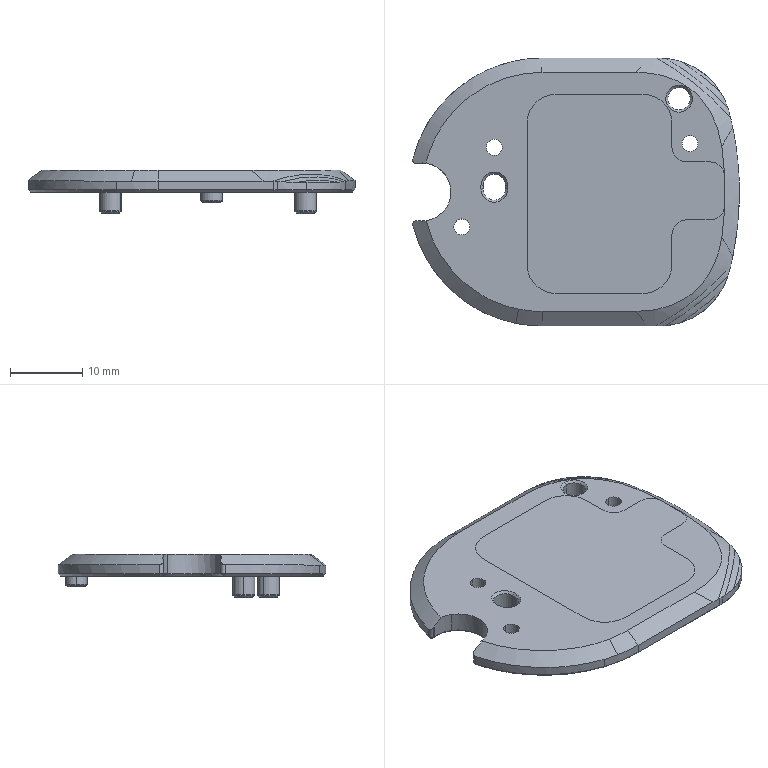NC program | NX | posted with a generic post | part box 45.101 x 36.973 x 6 mm
Lines 1809 to 2742 of 5084:
(ZLEVEL_PROFILE_1_COPY , TOOL : D3R0.5)
N3586 T18 M6
N3588 G54
N3590 G17 G0 G90 X-12.226 Y-12.18 S9500 M3
N3592 G43 Z30. H18
N3594 Z-2.01
N3596 G94 G1 Z-3.01 F1000.
N3598 X-12.477 Y-11.826
N3600 G3 X-12.75 Y-11.7 R0.3
N3602 G1 X-13.561 Y-11.776 F3000.
N3604 X-14.695 Y-11.793
N3606 X-14.752 Y-11.761
N3608 X-14.704 Y-12.064
N3610 X-14.705 Y-16.143
N3612 X-5.599 Y-16.003
N3614 G3 X-5.335 Y-15.728 R0.269
N3616 G1 X-5.334 Y-14.398
N3618 X-5.255 Y-13.594
N3620 X-5.37 Y-13.595 Z-3.019
N3622 X-5.415 Z-3.028
N3624 X-5.432 Y-14.398
N3626 Y-15.733
N3628 G2 X-5.601 Y-15.906 R0.171
N3630 G1 X-14.612 Y-16.044
N3632 X-14.608 Y-15.877
N3634 X-14.607 Y-12.131
N3636 X-14.614 Y-11.889
N3638 X-13.551 Y-11.873
N3640 X-12.739 Y-11.822
N3642 X-12.732 Y-11.89 Z-3.042
N3644 X-12.727 Y-11.939 Z-3.057
N3646 X-13.418 Y-11.959
N3648 X-13.54 Y-11.969
N3650 X-14.511 Y-11.984
N3652 X-14.512 Y-15.947
N3654 X-5.602 Y-15.81
N3656 X-5.56 Y-15.809
N3658 X-5.53 Y-15.778
N3660 X-5.528 Y-15.736
N3662 Y-14.398
N3664 X-5.509 Y-13.594
N3666 X-5.558 Y-13.595 Z-3.075
N3668 X-5.597 Z-3.094
N3670 X-5.619 Y-14.398
N3672 Y-15.719
N3674 X-14.42 Y-15.854
N3676 Y-12.074
N3678 X-13.529 Y-12.06
N3680 X-12.718 Y-12.035
N3682 X-12.712 Y-12.08 Z-3.117
N3684 X-12.707 Y-12.126 Z-3.139
N3686 X-13.418 Y-12.14
N3688 X-13.518 Y-12.146
N3690 X-14.333 Y-12.159
N3692 X-14.334 Y-15.766
N3694 X-5.706 Y-15.634
N3696 Y-14.398
N3698 X-5.686 Y-13.597
N3700 X-5.728 Z-3.166
N3702 X-5.772 Z-3.193
N3704 X-5.787 Y-14.398
N3706 Y-15.554
N3708 X-14.253 Y-15.684
N3710 X-14.252 Y-12.239
N3712 X-13.507 Y-12.227
N3714 X-12.697 Y-12.203
N3716 X-12.692 Y-12.246 Z-3.224
N3718 X-12.688 Y-12.283 Z-3.255
N3720 X-13.418 Y-12.296
N3722 X-13.496 Y-12.304
N3724 X-14.175 Y-12.315
N3726 X-14.176 Y-15.606
N3728 X-5.864 Y-15.478
N3730 Y-14.398
N3732 X-5.855 Y-14.33
N3734 X-5.844 Y-13.598
N3736 X-5.884 Z-3.29
N3738 X-5.917 Z-3.325
N3740 G2 X-5.934 Y-14.398 R6.646
N3742 G1 Y-15.409
N3744 X-14.105 Y-15.534
N3746 Y-12.384
N3748 X-13.485 Y-12.375
N3750 X-13.418 Y-12.371
N3752 X-12.679 Y-12.352
N3754 X-12.67 Y-12.39 Z-3.364
N3756 X-12.665 Y-12.412 Z-3.402
N3758 G3 X-13.475 Y-12.438 R18.194
N3760 G1 X-14.041 Y-12.447
N3762 Y-15.469
N3764 X-5.998 Y-15.346
N3766 Y-14.398
N3768 G3 X-5.981 Y-13.598 R6.688
N3770 G1 X-6.016 Z-3.444
N3772 X-6.044 Z-3.485
N3774 X-6.047 Y-14.33
N3776 X-6.053 Y-14.398
N3778 X-6.054 Y-15.291
N3780 X-13.986 Y-15.413
N3782 Y-12.501
N3784 X-13.466 Y-12.493
N3786 X-12.649 Y-12.469
N3788 X-12.633 Y-12.52 Z-3.571
N3790 X-12.69 Y-12.524
N3792 X-13.445 Y-12.536
N3794 X-13.458 Y-12.539
N3796 X-13.939 Y-12.547
N3798 X-13.94 Y-15.366
N3800 X-6.1 Y-15.246
N3802 Y-14.398
N3804 X-6.096 Y-14.33
N3806 Y-13.598
N3808 X-6.116 Z-3.614
N3810 X-6.138 Z-3.657
N3812 X-6.137 Y-14.33
N3814 X-6.135 Y-14.398
N3816 X-6.136 Y-15.211
N3818 X-13.904 Y-15.33
N3820 Y-12.582
N3822 X-13.451 Y-12.575
N3824 X-13.435 Y-12.577
N3826 X-12.69 Y-12.568
N3828 X-12.618 Y-12.564
N3830 X-12.603 Y-12.606 Z-3.738
N3832 X-12.69 Y-12.61
N3834 X-13.418 Y-12.617
N3836 X-13.429 Y-12.614
N3838 X-13.878 Y-12.621
N3840 Y-15.29
N3842 X-6.175 Y-15.172
N3844 Y-14.398
N3846 X-6.182 Y-14.33
N3848 X-6.183 Y-13.598
N3850 X-6.204 Z-3.768
N3852 X-6.224 Z-3.798
N3854 Y-14.33
N3856 X-6.217 Y-14.398
N3858 X-6.218 Y-15.13
N3860 X-13.864 Y-15.247
N3862 X-13.863 Y-12.663
N3864 X-13.405 Y-12.656
N3866 X-12.564 Y-12.649
N3868 X-12.508 Y-12.706 Z-3.859
N3870 X-13.371 Y-12.715
N3872 X-13.853 Y-12.723
N3874 Y-15.188
N3876 X-6.277 Y-15.071
N3878 Y-14.398
N3880 X-6.285 Y-14.33
N3882 Y-13.598
N3884 X-6.325 Z-3.886
N3886 X-6.367 Z-3.914
N3888 Y-14.33
N3890 X-6.355 Y-14.398
N3892 Y-14.995
N3894 X-13.847 Y-15.11
N3896 Y-12.8
N3898 X-13.323 Y-12.792
N3900 X-12.458 Y-12.786
N3902 X-12.351 Y-12.802 Z-3.926
N3904 X-12.243 Y-12.823 Z-3.938
N3906 X-12.136 Y-12.841 Z-3.951
N3908 X-12.222 Y-12.855
N3910 X-12.361 Y-12.869
N3912 X-12.448 Y-12.875
N3914 X-13.175 Y-12.889
N3916 X-13.265 Y-12.872
N3918 X-13.844 Y-12.881
N3920 Y-15.029
N3922 X-6.435 Y-14.916
N3924 Y-14.398
N3926 X-6.461 Y-14.33
N3928 X-6.45 Y-13.598
N3930 X-6.529 Y-13.602 Z-3.969
N3932 X-6.534 Y-14.33
N3934 X-6.5 Y-14.398
N3936 Y-14.851
N3938 X-13.844 Y-14.964
N3940 X-13.843 Y-12.946
N3942 X-13.213 Y-12.936
N3944 X-12.283 Y-12.95
N3946 G3 X-11.734 Y-12.785 R1.156
N3948 G1 X-11.72 Y-12.773
N3950 X-11.582 Y-12.722
N3952 X-11.587 Y-12.703
N3954 X-11.504 Y-12.759 Z-3.98
N3956 G2 X-12.142 Y-13.022 R0.839
N3958 G1 X-13.167 Y-12.989
N3960 X-13.843 Y-12.999
N3962 Y-14.911
N3964 X-6.553 Y-14.799
N3966 Y-14.398
N3968 G2 X-6.591 Y-13.594 R5.438
N3970 G3 X-6.734 Y-13.33 R0.3
N3972 G1 X-7.105 Y-13.103
N3974 Z-2.98
N3976 G0 Z30.
(ZLEVEL_PROFILE_1_COPY_COPY , TOOL : D3R0.5)
N3978 X11.743 Y-13.383
N3980 Z0.98
N3982 G1 Z-0.02 F1000.
N3984 X11.508 Y-12.976
N3986 G3 X11.248 Y-12.826 R0.3
N3988 G2 X8.967 Y-10.544 R2.282 F3000.
N3990 X11.248 Y-12.826 R-2.282
N3992 G1 Y-12.883 Z-0.036
N3994 Y-12.928 Z-0.053
N3996 G3 X13.632 Y-10.544 R2.384
N3998 X11.248 Y-12.928 R-2.384
N4000 G1 Y-12.978 Z-0.076
N4002 Y-13.02 Z-0.099
N4004 G2 X8.772 Y-10.544 R2.476
N4006 X11.248 Y-13.02 R-2.476
N4008 G1 Y-13.065 Z-0.128
N4010 Y-13.103 Z-0.157
N4012 G3 X13.808 Y-10.544 R2.559
N4014 X11.248 Y-13.103 R-2.559
N4016 G1 Y-13.142 Z-0.192
N4018 Y-13.177 Z-0.226
N4020 G2 X8.615 Y-10.544 R2.633
N4022 X11.248 Y-13.177 R-2.633
N4024 G1 Y-13.248 Z-0.297
N4026 G3 X13.952 Y-10.544 R2.704
N4028 X11.248 Y-13.248 R-2.704
N4030 G1 Y-13.318 Z-0.367
N4032 G2 X8.474 Y-10.544 R2.774
N4034 X11.248 Y-13.318 R-2.774
N4036 G1 Y-13.355 Z-0.404
N4038 Y-13.387 Z-0.441
N4040 G3 X14.091 Y-10.544 R2.843
N4042 X11.248 Y-13.387 R-2.843
N4044 G1 Y-13.418 Z-0.482
N4046 Y-13.445 Z-0.523
N4048 G2 X8.348 Y-10.544 R2.901
N4050 X11.248 Y-13.445 R-2.901
N4052 G1 Y-13.464 Z-0.558
N4054 Y-13.481 Z-0.593
N4056 G3 X14.185 Y-10.544 R2.937
N4058 X11.248 Y-13.481 R-2.937
N4060 G1 Y-13.495 Z-0.627
N4062 Y-13.508 Z-0.662
N4064 G2 X8.284 Y-10.544 R2.964
N4066 X11.248 Y-13.508 R-2.964
N4068 G1 Y-13.519 Z-0.696
N4070 Y-13.527 Z-0.731
N4072 G3 X14.232 Y-10.544 R2.983
N4074 X11.248 Y-13.527 R-2.983
N4076 G1 Y-13.534 Z-0.765
N4078 Y-13.539 Z-0.8
N4080 G2 X8.253 Y-10.544 R2.995
N4082 X11.248 Y-13.539 R-2.995
N4084 G3 X10.989 Y-13.689 R0.3
N4086 G1 X10.749 Y-14.104
N4088 Z0.2
N4090 G0 Z30.
N4092 X-18.519 Y-7.637
N4094 Z0.98
N4096 G1 Z-0.02 F1000.
N4098 X-18.111 Y-7.402
N4100 G3 X-17.961 Y-7.142 R0.3
N4102 G2 X-15.679 Y-4.86 R2.282 F3000.
N4104 X-17.961 Y-7.142 R-2.282
N4106 G1 X-18.019 Z-0.036
N4108 X-18.064 Z-0.053
N4110 G3 X-15.679 Y-9.526 R2.384
N4112 X-18.064 Y-7.142 R-2.384
N4114 G1 X-18.114 Z-0.076
N4116 X-18.156 Z-0.099
N4118 G2 X-15.679 Y-4.666 R2.476
N4120 X-18.156 Y-7.142 R-2.476
N4122 G1 X-18.2 Z-0.128
N4124 X-18.239 Z-0.157
N4126 G3 X-15.679 Y-9.702 R2.559
N4128 X-18.239 Y-7.142 R-2.559
N4130 G1 X-18.278 Z-0.192
N4132 X-18.313 Z-0.226
N4134 G2 X-15.679 Y-4.509 R2.633
N4136 X-18.313 Y-7.142 R-2.633
N4138 G1 X-18.383 Z-0.297
N4140 G3 X-15.679 Y-9.846 R2.704
N4142 X-18.383 Y-7.142 R-2.704
N4144 G1 X-18.454 Z-0.367
N4146 G2 X-15.679 Y-4.368 R2.775
N4148 X-18.454 Y-7.142 R-2.775
N4150 G1 X-18.49 Z-0.404
N4152 X-18.523 Z-0.441
N4154 G3 X-15.679 Y-9.985 R2.843
N4156 X-18.523 Y-7.142 R-2.843
N4158 G1 X-18.554 Z-0.482
N4160 X-18.58 Z-0.523
N4162 G2 X-15.679 Y-4.241 R2.901
N4164 X-18.58 Y-7.142 R-2.901
N4166 G1 X-18.6 Z-0.558
N4168 X-18.617 Z-0.593
N4170 G3 X-15.679 Y-10.079 R2.937
N4172 X-18.617 Y-7.142 R-2.937
N4174 G1 X-18.631 Z-0.627
N4176 X-18.644 Z-0.662
N4178 G2 X-15.679 Y-4.178 R2.964
N4180 X-18.644 Y-7.142 R-2.964
N4182 G1 X-18.654 Z-0.696
N4184 X-18.663 Z-0.731
N4186 G3 X-15.679 Y-10.126 R2.983
N4188 X-18.663 Y-7.142 R-2.983
N4190 G1 X-18.67 Z-0.765
N4192 X-18.675 Z-0.8
N4194 G2 X-15.679 Y-4.147 R2.995
N4196 X-18.675 Y-7.142 R-2.995
N4198 G3 X-18.825 Y-6.882 R0.3
N4200 G1 X-19.24 Y-6.643
N4202 Z0.2
N4204 G0 Z30.
(ZLEVEL_PROFILE_1_COPY_COPY_COPY , TOOL : D3R0.5)
N4206 X-3.201 Y18.824
N4208 Z-0.52
N4210 G1 Z-1.52 F1000.
N4212 X-2.966 Y18.417
N4214 G3 X-2.707 Y18.267 R0.3
N4216 G2 X-0.425 Y15.985 R2.282 F3000.
N4218 X-2.707 Y18.267 R-2.282
N4220 G1 Y18.324 Z-1.536
N4222 Y18.369 Z-1.553
N4224 G3 X-5.091 Y15.985 R2.384
N4226 X-2.707 Y18.369 R-2.384
N4228 G1 Y18.419 Z-1.576
N4230 Y18.461 Z-1.599
N4232 G2 X-0.231 Y15.985 R2.476
N4234 X-2.707 Y18.461 R-2.476
N4236 G1 Y18.506 Z-1.628
N4238 Y18.544 Z-1.657
N4240 G3 X-5.266 Y15.985 R2.559
N4242 X-2.707 Y18.544 R-2.559
N4244 G1 Y18.583 Z-1.692
N4246 Y18.618 Z-1.726
N4248 G2 X-0.074 Y15.985 R2.633
N4250 X-2.707 Y18.618 R-2.633
N4252 G1 Y18.689 Z-1.797
N4254 G3 X-5.41 Y15.985 R2.704
N4256 X-2.707 Y18.689 R-2.704
N4258 G1 Y18.759 Z-1.867
N4260 G2 X0.068 Y15.985 R2.774
N4262 X-2.707 Y18.759 R-2.774
N4264 G1 Y18.796 Z-1.904
N4266 Y18.828 Z-1.941
N4268 G3 X-5.55 Y15.985 R2.843
N4270 X-2.707 Y18.828 R-2.843
N4272 G1 Y18.859 Z-1.982
N4274 Y18.886 Z-2.023
N4276 G2 X0.194 Y15.985 R2.901
N4278 X-2.707 Y18.886 R-2.901
N4280 G1 Y18.905 Z-2.058
N4282 Y18.922 Z-2.093
N4284 G3 X-5.644 Y15.985 R2.937
N4286 X-2.707 Y18.922 R-2.937
N4288 G1 Y18.937 Z-2.127
N4290 Y18.949 Z-2.162
N4292 G2 X0.258 Y15.985 R2.964
N4294 X-2.707 Y18.949 R-2.964
N4296 G1 Y18.96 Z-2.196
N4298 Y18.968 Z-2.231
N4300 G3 X-5.69 Y15.985 R2.983
N4302 X-2.707 Y18.968 R-2.983
N4304 G1 Y18.975 Z-2.265
N4306 Y18.98 Z-2.3
N4308 G2 X0.289 Y15.985 R2.995
N4310 X-2.707 Y18.98 R-2.995
N4312 G3 X-2.447 Y19.13 R0.3
N4314 G1 X-2.207 Y19.545
N4316 Z-1.3
N4318 G0 Z30.
(FIXED_CONTOUR , TOOL : D3R0.5)
N4320 X-12.11 Y-12.283
N4322 Z0.
N4324 G1 Z-3.651 F1000.
N4326 G2 X-12.234 Y-12.01 R0.3
N4328 G1 X-12.229 Y-11.962 Z-3.584 F2500.
N4330 X-12.201 Y-11.849 Z-3.494
N4332 X-12.145 Y-11.593 Z-3.363
N4334 X-12.132 Y-11.319 Z-3.254
N4336 X-12.149 Y-11.088 Z-3.182
N4338 X-12.19 Y-10.835 Z-3.124
N4340 X-12.25 Y-10.577 Z-3.086
N4342 X-12.295 Y-10.368 Z-3.077
N4344 X-12.296 Y-9.711 Z-3.086
N4346 Y-8.106
N4348 Y-6.502
N4350 X-12.292 Y-6.1 Z-3.088
N4352 X-12.295 Y-5.541 Z-3.096
N4354 X-12.362 Y-5.173 Z-3.093
N4356 X-12.473 Y-4.819 Z-3.09
N4358 X-12.626 Y-4.482 Z-3.089
N4360 X-12.82 Y-4.166 Z-3.087
N4362 X-13.051 Y-3.875
N4364 X-13.318 Y-3.613 Z-3.086
N4366 X-13.613 Y-3.389 Z-3.087
N4368 X-13.931 Y-3.203 Z-3.088
N4370 X-14.269 Y-3.057 Z-3.089
N4372 X-14.624 Y-2.953 Z-3.091
N4374 X-14.99 Y-2.893 Z-3.093
N4376 X-15.325 Y-2.882
N4378 X-16.93 Y-2.894 Z-3.086
N4380 X-18.534
N4382 X-18.717 Y-2.893 Z-3.077
N4384 X-18.881 Y-2.841 Z-3.079
N4386 X-19.034 Y-2.765 Z-3.082
N4388 X-19.173 Y-2.666 Z-3.084
N4390 X-19.296 Y-2.546 Z-3.085
N4392 X-19.398 Y-2.409 Z-3.086
N4394 X-19.476 Y-2.258
N4396 X-19.53 Y-2.097
N4398 X-19.559 Y-1.929 Z-3.085
N4400 X-19.56 Y-1.619 Z-3.086
N4402 Y-0.817
N4404 Y0.788
N4406 X-19.559 Y1.59
N4408 X-19.556 Y2.252
N4410 X-19.527 Y2.42 Z-3.085
N4412 X-19.474 Y2.581 Z-3.083
N4414 X-19.395 Y2.732 Z-3.081
N4416 X-19.293 Y2.871 Z-3.078
N4418 X-19.168 Y2.994 Z-3.076
N4420 X-19.026 Y3.095 Z-3.072
N4422 X-18.869 Y3.173 Z-3.068
N4424 X-18.699 Y3.215 Z-3.069
N4426 X-18.465 Y3.198 Z-3.086
N4428 X-18.064 Y3.197
N4430 X-17.262
N4432 X-15.657 Y3.194 Z-3.088
N4434 X-15.22 Y3.157 Z-3.11
N4436 X-14.846 Y3.194 Z-3.105
N4438 X-14.48 Y3.275 Z-3.1
N4440 X-14.129 Y3.4 Z-3.096
N4442 X-13.797 Y3.566 Z-3.093
N4444 X-13.488 Y3.771 Z-3.091
N4446 X-13.204 Y4.014 Z-3.089
N4448 X-12.953 Y4.291 Z-3.087
N4450 X-12.74 Y4.593
N4452 X-12.566 Y4.917 Z-3.086
N4454 X-12.433 Y5.26 Z-3.087
N4456 X-12.342 Y5.618 Z-3.088
N4458 X-12.296 Y5.986 Z-3.089
N4460 Y6.472 Z-3.086
N4462 Y8.077
N4464 X-12.297 Y9.628 Z-3.084
N4466 X-12.271 Y9.903
N4468 X-12.22 Y10.174 Z-3.085
N4470 X-12.145 Y10.439
N4472 X-12.047 Y10.695
N4474 X-11.926 Y10.942 Z-3.086
N4476 X-11.783 Y11.177
N4478 G2 X-9.756 Y12.49 R3.06
N4480 G1 X-9.482 Y12.524 Z-3.085
N4482 X-7.973 Y12.53 Z-3.086
N4484 X-6.368
N4486 X-4.764
N4488 X-3.159
N4490 X-1.555
N4492 X0.05
N4494 X1.654
N4496 X2.457
N4498 G2 X3.899 Y12.306 R3.332
N4500 G1 X4.148 Y12.191
N4502 X4.387 Y12.054
N4504 X4.613 Y11.895
N4506 X4.825 Y11.716
N4508 X5.021 Y11.517
N4510 X5.197 Y11.303 Z-3.085
N4512 X5.351 Y11.075
N4514 X5.485 Y10.835 Z-3.084
N4516 X5.596 Y10.584
N4518 X5.684 Y10.324 Z-3.083
N4520 X5.749 Y10.057
N4522 X5.79 Y9.784 Z-3.082
N4524 X5.796 Y9.501 Z-3.086
N4526 Y3.082
N4528 Y-9.754
N4530 Y-10.115
N4532 X5.774 Y-10.39
N4534 G2 X4.765 Y-12.301 R3.06
N4536 G1 X4.55 Y-12.475 Z-3.085
N4538 X4.321 Y-12.628
N4540 X4.08 Y-12.759
N4542 X3.829 Y-12.868 Z-3.084
N4544 X3.568 Y-12.955
N4546 X3.3 Y-13.018 Z-3.083
N4548 X3.026 Y-13.057 Z-3.082
N4550 X2.734 Y-13.061 Z-3.086
N4552 X1.932
N4554 X0.327
N4556 X-1.277
N4558 X-2.882
N4560 X-3.684
N4562 X-3.968 Y-13.051 Z-3.091
N4564 X-4.195 Y-13.029 Z-3.104
N4566 X-4.51 Y-13.002 Z-3.144
N4568 X-4.782 Y-13.014 Z-3.195
N4570 X-5.038 Y-13.05 Z-3.266
N4572 X-5.297 Y-13.124 Z-3.356
N4574 X-5.434 Y-13.185 Z-3.409
N4576 X-5.579 Y-13.272 Z-3.468
N4578 X-5.733 Y-13.394 Z-3.533
N4580 X-5.895 Y-13.574 Z-3.608
N4582 X-5.886 Y-13.518 Z-3.663
N4584 X-5.87 Y-13.462 Z-3.718
N4586 X-5.828 Y-13.299 Z-3.868
N4588 X-5.781 Y-13.19 Z-3.945
N4590 X-5.722 Y-13.1 Z-3.998
N4592 X-5.646 Y-13.034 Z-4.016
N4594 X-5.6 Y-13.006 Z-4.009
N4596 X-5.673 Y-13.035 Z-4.04
N4598 X-5.754 Y-13.061 Z-4.066
N4600 X-7.278
N4602 X-8.882
N4604 X-9.547 Y-13.047
N4606 X-9.82 Y-13.008
N4608 X-10.088 Y-12.945
N4610 X-10.349 Y-12.858
N4612 X-10.602 Y-12.748 Z-4.065
N4614 X-10.843 Y-12.615
N4616 X-11.072 Y-12.462 Z-4.064
N4618 X-11.286 Y-12.288
N4620 X-11.484 Y-12.095 Z-4.063
N4622 X-11.765 Y-11.749 Z-4.062
N4624 X-11.823 Y-11.675 Z-4.059
N4626 X-11.82 Y-11.549 Z-3.962
N4628 X-11.822 Y-11.483 Z-3.884
N4630 X-11.871 Y-11.652 Z-3.95
N4632 X-11.907 Y-11.744 Z-3.966
N4634 X-11.985 Y-11.89 Z-3.946
N4636 X-12.005 Y-11.901 Z-3.926
N4638 X-12.026 Y-11.933 Z-3.92
N4640 X-12.108 Y-11.981 Z-3.847
N4642 X-12.179 Y-12.005 Z-3.758
N4644 X-12.21 Y-12.015 Z-3.713
N4646 X-12.234 Y-12.009 Z-3.65
N4648 X-12.207 Y-11.983 Z-3.658
N4650 X-12.184 Y-11.988 Z-3.722
N4652 X-12.153 Y-11.977 Z-3.766
N4654 X-12.083 Y-11.952 Z-3.855
N4656 X-12.047 Y-11.937 Z-3.896
N4658 X-12.014 Y-11.916 Z-3.926
N4660 X-11.985 Y-11.889 Z-3.946
N4662 X-11.962 Y-11.857 Z-3.956
N4664 X-11.924 Y-11.786 Z-3.968
N4666 X-11.888 Y-11.716 Z-3.978
N4668 X-11.865 Y-11.66 Z-3.971
N4670 X-11.839 Y-11.589 Z-3.956
N4672 X-11.816 Y-11.487 Z-3.905
N4674 X-11.806 Y-11.439 Z-3.878
N4676 X-11.801 Y-11.433 Z-3.887
N4678 X-11.799 Y-11.475 Z-3.942
N4680 X-11.796 Y-11.516 Z-3.989
N4682 X-11.797 Y-11.586 Z-4.044
N4684 X-11.796 Y-11.642 Z-4.082
N4686 X-11.47 Y-12.053 Z-4.086
N4688 X-11.274 Y-12.246
N4690 X-11.062 Y-12.42 Z-4.087
N4692 X-10.836 Y-12.574
N4694 X-10.596 Y-12.707 Z-4.088
N4696 X-10.345 Y-12.818
N4698 X-10.086 Y-12.906
N4700 X-9.819 Y-12.969 Z-4.089
N4702 X-9.548 Y-13.008
N4704 X-8.885 Y-13.023
N4706 X-7.323
N4708 X-5.761
N4710 X-5.723
N4712 X-5.67 Y-13.007 Z-4.074
N4714 X-5.617 Y-12.988 Z-4.054
N4716 X-5.641 Y-13.004
N4718 X-5.723 Y-13.067 Z-4.039
N4720 X-5.786 Y-13.157 Z-3.987
N4722 X-5.834 Y-13.269 Z-3.91
N4724 X-5.886 Y-13.488 Z-3.713
N4726 X-5.897 Y-13.54 Z-3.657
N4728 X-5.734 Y-13.359 Z-3.583
N4730 X-5.58 Y-13.235 Z-3.517
N4732 X-5.435 Y-13.147 Z-3.458
N4734 X-5.298 Y-13.085 Z-3.404
N4736 X-5.039 Y-13.008 Z-3.311
N4738 X-4.785 Y-12.971 Z-3.236
N4740 X-4.516 Y-12.959 Z-3.18
N4742 X-4.181 Y-12.988 Z-3.13
N4744 X-3.961 Y-13.012 Z-3.115
N4746 X-3.698 Y-13.023 Z-3.109
N4748 X-2.897
N4750 X0.306
N4752 X1.908
N4754 X2.708
N4756 X2.999 Y-13.02 Z-3.105
N4758 X3.272 Y-12.983
N4760 X3.539 Y-12.923 Z-3.106
N4762 X3.799 Y-12.838 Z-3.107
N4764 X4.049 Y-12.731
N4766 X4.29 Y-12.602 Z-3.108
N4768 X4.518 Y-12.451
N4770 X4.733 Y-12.278
N4772 X4.933 Y-12.086 Z-3.109
N4774 G3 X5.757 Y-10.105 R3.02
N4776 G1 X5.758 Y-9.745
N4778 Y3.067
N4780 Y9.474
N4782 X5.753 Y9.755 Z-3.104
N4784 X5.715 Y10.028 Z-3.105
N4786 X5.652 Y10.294 Z-3.106
N4788 X5.566 Y10.553
N4790 X5.457 Y10.803 Z-3.107
N4792 X5.326 Y11.043
N4794 X5.173 Y11.27 Z-3.108
N4796 X4.999 Y11.484
N4798 X4.805 Y11.682 Z-3.109
N4800 X4.595 Y11.861
N4802 G3 X2.819 Y12.492 R3.02
N4804 G1 X2.449
N4806 X1.648
N4808 X0.047
N4810 X-3.156
N4812 X-6.36
N4814 X-7.961
N4816 X-9.466 Y12.486 Z-3.108
N4818 X-9.739 Y12.453
N4820 X-10.007 Y12.396 Z-3.109
N4822 X-10.267 Y12.315
N4824 G3 X-11.897 Y10.915 R3.02
N4826 G1 X-12.016 Y10.669 Z-3.108
N4828 X-12.113 Y10.414
N4830 X-12.186 Y10.15 Z-3.107
N4832 X-12.235 Y9.88
N4834 X-12.259 Y9.607 Z-3.106
N4836 X-12.257 Y8.059 Z-3.109
N4838 Y6.457
N4840 X-12.259 Y5.971 Z-3.112
N4842 X-12.306 Y5.603 Z-3.11
N4844 X-12.398 Y5.245 Z-3.109
N4846 X-12.531 Y4.901
N4848 X-12.705 Y4.576
N4850 X-12.918 Y4.273 Z-3.11
N4852 X-13.169 Y3.995 Z-3.111
N4854 X-13.452 Y3.751 Z-3.113
N4856 X-13.761 Y3.543 Z-3.116
N4858 X-14.093 Y3.375 Z-3.119
N4860 X-14.443 Y3.248 Z-3.123
N4862 X-14.808 Y3.164 Z-3.128
N4864 X-15.182 Y3.124 Z-3.133
N4866 X-15.619 Y3.156 Z-3.111
N4868 X-17.22 Y3.159 Z-3.109
N4870 X-18.021
N4872 X-18.421
N4874 X-18.653 Y3.179 Z-3.092
N4876 X-18.822 Y3.143 Z-3.091
N4878 X-18.979 Y3.072 Z-3.095
N4880 X-19.122 Y2.977 Z-3.098
N4882 X-19.248 Y2.86 Z-3.101
N4884 X-19.352 Y2.725 Z-3.104
N4886 X-19.432 Y2.578 Z-3.106
N4888 X-19.488 Y2.419 Z-3.108
N4890 X-19.517 Y2.254 Z-3.109
N4892 X-19.521 Y1.594
N4894 Y0.793
N4896 Y-0.808
N4898 X-19.522 Y-1.609
N4900 X-19.521 Y-1.918 Z-3.108
N4902 X-19.494 Y-2.084 Z-3.109
N4904 X-19.441 Y-2.243
N4906 X-19.363 Y-2.391
N4908 X-19.262 Y-2.526 Z-3.108
N4910 X-19.139 Y-2.644 Z-3.106
N4912 X-19. Y-2.739 Z-3.105
N4914 X-18.848 Y-2.811 Z-3.102
N4916 X-18.685 Y-2.858 Z-3.099
N4918 X-18.504 Y-2.856 Z-3.109
N4920 X-16.902
N4922 X-15.301 Y-2.845 Z-3.116
N4924 X-14.966 Y-2.859
N4926 X-14.599 Y-2.921 Z-3.114
N4928 X-14.245 Y-3.026 Z-3.112
N4930 X-13.906 Y-3.173 Z-3.11
N4932 X-13.588 Y-3.359 Z-3.109
N4934 X-13.293 Y-3.585
N4936 X-13.025 Y-3.847
N4938 X-12.793 Y-4.138 Z-3.11
N4940 X-12.598 Y-4.454 Z-3.111
N4942 X-12.444 Y-4.791 Z-3.113
N4944 X-12.331 Y-5.145 Z-3.116
N4946 X-12.261 Y-5.512 Z-3.119
N4948 X-12.254 Y-6.072 Z-3.111
N4950 X-12.257 Y-6.472 Z-3.109
N4952 Y-8.074
N4954 Y-9.675
N4956 X-12.259 Y-10.331 Z-3.099
N4958 X-12.215 Y-10.539 Z-3.109
N4960 X-12.155 Y-10.799 Z-3.146
N4962 X-12.116 Y-11.052 Z-3.202
N4964 X-12.101 Y-11.285 Z-3.272
N4966 X-12.116 Y-11.561 Z-3.377
N4968 X-12.173 Y-11.821 Z-3.503
N4970 X-12.202 Y-11.935 Z-3.593
N4972 X-12.207 Y-11.984 Z-3.659
N4974 X-12.181 Y-11.958 Z-3.669
N4976 X-12.175 Y-11.902 Z-3.595
N4978 X-12.146 Y-11.78 Z-3.503
N4980 X-12.088 Y-11.508 Z-3.381
N4982 X-12.072 Y-11.233 Z-3.284
N4984 X-12.086 Y-11.003 Z-3.221
N4986 X-12.124 Y-10.756 Z-3.169
N4988 X-12.181 Y-10.506 Z-3.134
N4990 X-12.222 Y-10.302 Z-3.125
N4992 X-12.221 Y-9.64 Z-3.134
N4994 Y-8.041
N4996 Y-6.443
N4998 X-12.219 Y-6.037 Z-3.135
N5000 X-12.233 Y-5.472 Z-3.143
N5002 X-12.305 Y-5.108 Z-3.14
N5004 X-12.42 Y-4.756 Z-3.137
N5006 X-12.575 Y-4.422 Z-3.136
N5008 X-12.77 Y-4.108 Z-3.135
N5010 X-13.002 Y-3.819 Z-3.134
N5012 X-13.268 Y-3.558
N5014 X-13.562 Y-3.333
N5016 X-13.878 Y-3.147 Z-3.135
N5018 X-14.214 Y-2.999 Z-3.136
N5020 X-14.567 Y-2.892 Z-3.138
N5022 X-14.931 Y-2.828 Z-3.14
N5024 X-15.266 Y-2.812
N5026 X-16.875 Y-2.82 Z-3.134
N5028 X-18.474
N5030 X-18.593 Y-2.828 Z-3.125
N5032 X-18.665 Y-2.821
N5034 X-18.825 Y-2.778 Z-3.127
N5036 X-18.975 Y-2.71 Z-3.13
N5038 X-19.111 Y-2.618 Z-3.131
N5040 X-19.232 Y-2.505 Z-3.133
N5042 X-19.331 Y-2.374
N5044 X-19.408 Y-2.229 Z-3.134
N5046 X-19.459 Y-2.073 Z-3.133
N5048 X-19.485 Y-1.911
N5050 Y-1.599 Z-3.134
N5052 Y-0.8
N5054 Y0.799
N5056 Y1.598
N5058 X-19.48 Y2.253 Z-3.133
N5060 X-19.451 Y2.414 Z-3.132
N5062 X-19.395 Y2.568 Z-3.131
N5064 X-19.316 Y2.711 Z-3.129
N5066 X-19.212 Y2.841 Z-3.126
N5068 X-19.087 Y2.953 Z-3.124
N5070 X-18.947 Y3.042 Z-3.121
N5072 X-18.792 Y3.107 Z-3.117
N5074 X-18.617 Y3.141
N5076 X-18.378 Y3.123 Z-3.134
N5078 X-17.978
N5080 X-17.179
N5082 X-15.575 Y3.122 Z-3.135
N5084 X-15.126 Y3.097 Z-3.155
N5086 X-14.755 Y3.141 Z-3.15
N5088 X-14.393 Y3.229 Z-3.146
N5090 X-14.046 Y3.359 Z-3.143
N5092 X-13.718 Y3.529 Z-3.14
N5094 X-13.412 Y3.738 Z-3.138
N5096 X-13.132 Y3.982 Z-3.136
N5098 X-12.883 Y4.26 Z-3.135
N5100 X-12.671 Y4.562 Z-3.134
N5102 X-12.498 Y4.886
N5104 X-12.365 Y5.227
N5106 X-12.273 Y5.584 Z-3.135
N5108 X-12.225 Y5.95 Z-3.136
N5110 X-12.221 Y6.442 Z-3.134
N5112 Y8.041
N5114 X-12.223 Y9.589 Z-3.131
N5116 X-12.2 Y9.862 Z-3.132
N5118 X-12.153 Y10.13
N5120 X-12.081 Y10.393
N5122 X-11.986 Y10.647 Z-3.133
N5124 X-11.868 Y10.891
N5126 X-11.728 Y11.125
N5128 G2 X-9.726 Y12.419 R2.981
N5130 G1 X-9.454 Y12.45
N5132 X-7.949 Y12.456 Z-3.134
N5134 X-6.351
N5136 X-3.154
N5138 X0.044
N5140 X1.642
N5142 X2.441
N5144 G2 X3.872 Y12.236 R3.295
N5146 G1 X4.118 Y12.122
N5148 X4.353 Y11.987
N5150 X4.576 Y11.829 Z-3.133
N5152 X4.785 Y11.651
N5154 X4.977 Y11.453
N5156 X5.149 Y11.24
N5158 X5.3 Y11.014 Z-3.132
N5160 X5.429 Y10.776
N5162 X5.536 Y10.527 Z-3.131
N5164 X5.62 Y10.269
N5166 X5.681 Y10.004 Z-3.13
N5168 X5.717 Y9.733 Z-3.129
N5170 X5.722 Y9.447 Z-3.134
N5172 Y3.052
N5174 Y-9.736
N5176 X5.721 Y-10.098 Z-3.133
N5178 X5.701 Y-10.369
N5180 G2 X4.703 Y-12.256 R2.981
N5182 G1 X4.49 Y-12.426
N5184 X4.262 Y-12.575 Z-3.132
N5186 X4.023 Y-12.703
N5188 X3.774 Y-12.808
N5190 X3.515 Y-12.89 Z-3.131
N5192 X3.25 Y-12.949 Z-3.13
N5194 X2.979 Y-12.983
N5196 X2.683 Y-12.987 Z-3.134
N5198 X1.884
N5200 X0.285
N5202 X-2.912
N5204 X-3.711
N5206 X-3.851 Y-12.98 Z-3.136
N5208 X-4.009 Y-12.964 Z-3.144
N5210 X-4.19 Y-12.946 Z-3.161
N5212 X-4.434 Y-12.93 Z-3.194
N5214 X-4.572 Y-12.929 Z-3.219
N5216 X-4.823 Y-12.941 Z-3.282
N5218 X-5.061 Y-12.978 Z-3.36
N5220 X-5.303 Y-13.052 Z-3.455
N5222 X-6.091 Y-12.987 Z-4.114
N5224 X-8.889
N5226 X-9.548 Y-12.972
N5228 X-9.817 Y-12.933 Z-4.113
N5230 X-10.082 Y-12.869
N5232 X-10.339 Y-12.781
N5234 X-10.588 Y-12.67
N5236 X-10.826 Y-12.537 Z-4.112
N5238 X-11.05 Y-12.383
N5240 X-11.26 Y-12.209 Z-4.111
N5242 X-11.453 Y-12.016
N5244 X-11.718 Y-11.68 Z-4.11
N5246 X-11.77 Y-11.61 Z-4.108
N5248 X-11.774 Y-11.494 Z-4.023
N5250 X-11.782 Y-11.448 Z-3.96
N5252 X-11.843 Y-11.644 Z-4.
N5254 X-11.899 Y-11.761 Z-3.991
N5256 X-11.94 Y-11.835 Z-3.974
N5258 X-11.959 Y-11.847 Z-3.953
N5260 X-11.98 Y-11.878 Z-3.945
N5262 X-12.06 Y-11.928 Z-3.868
N5264 X-12.129 Y-11.952 Z-3.776
N5266 X-12.159 Y-11.962 Z-3.731
N5268 X-12.182 Y-11.957 Z-3.667
N5270 X-12.157 Y-11.931 Z-3.678
N5272 X-12.134 Y-11.936 Z-3.742
N5274 X-12.105 Y-11.927 Z-3.788
N5276 X-12.037 Y-11.905 Z-3.882
N5278 X-12.003 Y-11.891 Z-3.923
N5280 X-11.971 Y-11.872 Z-3.955
N5282 X-11.942 Y-11.847 Z-3.978
N5284 X-11.918 Y-11.816 Z-3.994
N5286 X-11.864 Y-11.724 Z-4.025
N5288 X-11.83 Y-11.656 Z-4.034
N5290 X-11.795 Y-11.562 Z-4.03
N5292 X-11.769 Y-11.446 Z-3.995
N5294 X-11.753 Y-11.482 Z-4.064
N5296 X-11.745 Y-11.581 Z-4.136
N5298 X-11.734 Y-11.595 Z-4.137
N5300 X-11.436 Y-11.982 Z-4.138
N5302 X-11.245 Y-12.174
N5304 X-11.038 Y-12.348 Z-4.139
N5306 X-10.816 Y-12.502
N5308 X-10.58 Y-12.635
N5310 X-10.333 Y-12.746 Z-4.14
N5312 X-10.078 Y-12.834
N5314 X-9.815 Y-12.898
N5316 X-9.548 Y-12.937
N5318 X-8.892 Y-12.952
N5320 X-7.298
N5322 X-5.705
N5324 X-5.671
N5326 X-5.625 Y-12.939 Z-4.125
N5328 X-5.643 Y-12.95
N5330 X-5.695 Y-12.987 Z-4.114
N5332 X-5.701 Y-12.991 Z-4.111
N5334 X-5.744 Y-13.045 Z-4.076
N5336 X-5.761 Y-13.077 Z-4.054
N5338 X-5.796 Y-13.168 Z-3.984
N5340 X-5.824 Y-13.35 Z-3.794
N5342 X-5.829 Y-13.391 Z-3.74
N5344 X-5.683 Y-13.25 Z-3.675
N5346 X-5.55 Y-13.15 Z-3.616
N5348 X-5.311 Y-13.021 Z-3.506
N5350 X-5.091 Y-12.952 Z-3.41
N5352 X-4.876 Y-12.918 Z-3.329
N5354 X-4.65 Y-12.907 Z-3.26
N5356 X-4.514 Y-12.91 Z-3.22
N5358 X-4.402 Y-12.924 Z-3.19
N5360 X-4.227 Y-12.949 Z-3.164
N5362 X-3.725 Y-12.952 Z-3.16
N5364 X-2.927
N5366 X0.264
N5368 X1.859
N5370 X2.657
N5372 X2.96 Y-12.949 Z-3.157
N5374 X3.23 Y-12.916 Z-3.158
N5376 X3.494 Y-12.859
N5378 X3.75 Y-12.779 Z-3.159
N5380 X3.999 Y-12.676
N5382 X4.237 Y-12.55
N5384 X4.463 Y-12.402 Z-3.16
N5386 X4.676 Y-12.234
N5388 X4.874 Y-12.045
N5390 G3 X5.687 Y-10.091 R2.944
N5392 G1 Y-9.727
N5394 Y3.037
N5396 Y9.42
N5398 X5.682 Y9.714 Z-3.157
N5400 X5.648 Y9.983 Z-3.158
N5402 X5.59 Y10.247
N5404 X5.508 Y10.503
N5406 X5.402 Y10.75 Z-3.159
N5408 X5.275 Y10.988
N5410 X5.126 Y11.213
N5412 X4.956 Y11.425 Z-3.16
N5414 X4.766 Y11.622
N5416 G3 X2.806 Y12.421 R2.944
N5418 G1 X2.434 Y12.422
N5420 X1.636
N5422 X0.041
N5424 X-1.555
N5426 X-3.151
N5428 X-6.342